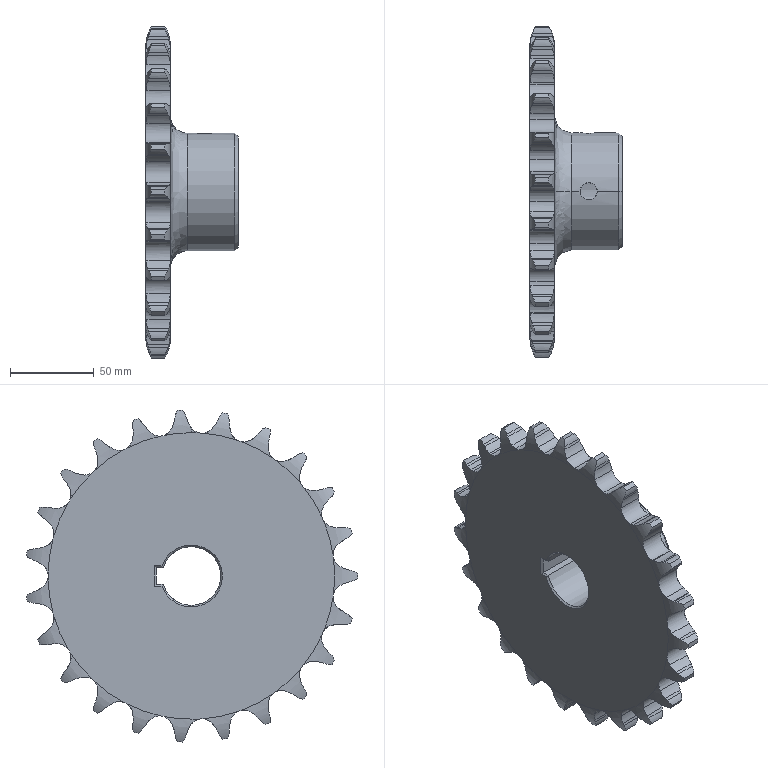Part | STEP file | 1 solid | 273 faces | box 55.024 x 197.271 x 197.721 mm | volume 475495 mm3 | cylinder 157 | plane 61 | spline 50 | cone 5 | commonest cylinder face diameters 23.032 x49 41.467 x48 16.059 x30 198 x23 10.2 x4 70 x2